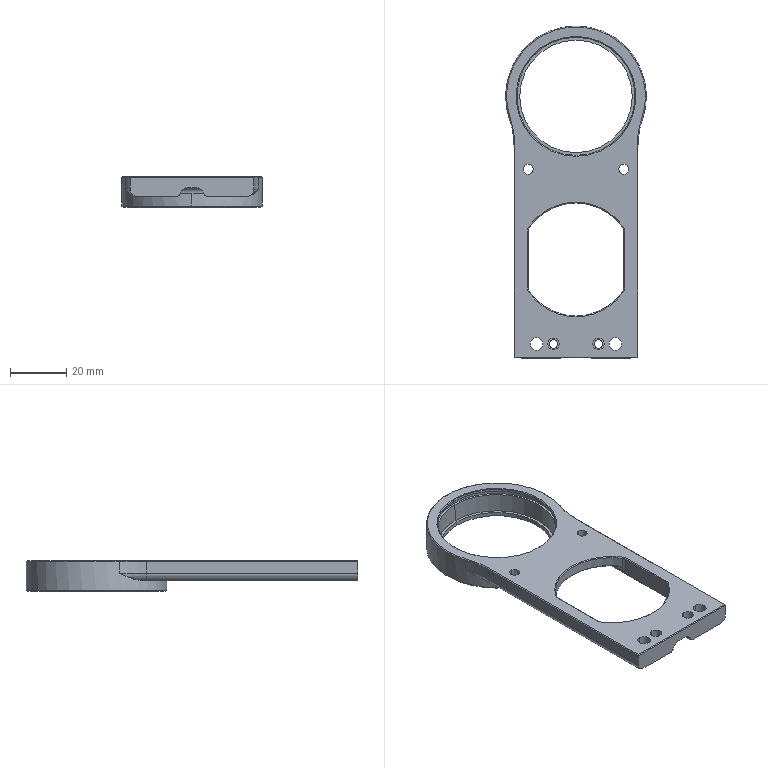NC program | NX | posted with a generic post | part box 50 x 118 x 11 mm
Lines 1103 to 2100 of 9841:
(ZLEVEL_PROFILE_1_COPY , TOOL : D3R0.5)
N2168 T18 M6
N2170 G54
N2172 G17 G0 G90 X65.824 Y-6.743 S9500 M3
N2174 G43 Z30. H18
N2176 Z-1.012
N2178 G94 G1 Z-4.012 F1000.
N2180 X65.888 Y-6.726
N2182 G3 X66.956 Y-4.893 R1.5
N2184 G2 X66.711 Y-3.914 R38.728 F2500.
N2186 G1 X66.672 Y-3.67
N2188 X66.526 Y-2.446
N2190 X66.5 Y-2.202
N2192 X66.495 Y-2.079
N2194 X66.436 Y-0.489
N2196 X66.429 Y-0.245
N2198 X66.5 Y2.202
N2200 X66.526 Y2.446
N2202 X66.663 Y3.595
N2204 G2 X66.812 Y4.34 R4.831
N2206 G3 X67.039 Y5.31 R10.605
N2208 G1 X67.047 Y5.352 Z-4.025
N2210 G2 X66.812 Y4.342 R11.706
N2212 G3 X66.662 Y3.59 R4.971
N2214 G1 X66.526 Y2.446
N2216 X66.5 Y2.202
N2218 X66.429 Y-0.245
N2220 X66.436 Y-0.489
N2222 X66.495 Y-2.079
N2224 X66.5 Y-2.202
N2226 X66.526 Y-2.446
N2228 X66.672 Y-3.67
N2230 X66.711 Y-3.914
N2232 G3 X66.956 Y-4.893 R23.385
N2234 G1 X66.971 Y-4.975 Z-4.03
N2236 X66.987 Y-5.056 Z-4.034
N2238 X67.003 Y-5.138 Z-4.039
N2240 G3 X66.837 Y-4.45 R8.75
N2242 G2 X66.658 Y-3.557 R5.791
N2244 G1 X66.526 Y-2.446
N2246 X66.5 Y-2.202
N2248 X66.495 Y-2.079
N2250 X66.436 Y-0.489
N2252 X66.429 Y-0.245
N2254 X66.5 Y2.202
N2256 X66.526 Y2.446
N2258 X66.672 Y3.67
N2260 X66.711 Y3.914
N2262 G2 X66.953 Y4.893 R19.424
N2264 G1 X67.056 Y5.396
N2266 X67.069 Y5.454 Z-4.057
N2268 G2 X66.829 Y4.433 R13.052
N2270 G3 X66.663 Y3.593 R5.641
N2272 G1 X66.526 Y2.446
N2274 X66.5 Y2.202
N2276 X66.429 Y-0.245
N2278 X66.436 Y-0.489
N2280 X66.495 Y-2.079
N2282 X66.5 Y-2.202
N2284 X66.526 Y-2.446
N2286 X66.664 Y-3.605
N2288 G3 X66.82 Y-4.399 R5.379
N2290 G2 X67.003 Y-5.138 R13.895
N2292 G1 Z-4.08
N2294 G2 X66.711 Y-3.914 R40.513
N2296 G1 X66.672 Y-3.67
N2298 X66.526 Y-2.446
N2300 X66.5 Y-2.202
N2302 X66.495 Y-2.079
N2304 X66.436 Y-0.489
N2306 X66.429 Y-0.245
N2308 X66.5 Y2.202
N2310 X66.526 Y2.446
N2312 X66.672 Y3.67
N2314 X66.711 Y3.914
N2316 X66.895 Y4.704
N2318 X66.946 Y4.893
N2320 X67.084 Y5.528
N2322 X67.104 Y5.618 Z-4.108
N2324 X67.002 Y5.138
N2326 G3 X66.711 Y3.914 R30.653
N2328 G1 X66.672 Y3.67
N2330 X66.526 Y2.446
N2332 X66.5 Y2.202
N2334 X66.429 Y-0.245
N2336 X66.436 Y-0.489
N2338 X66.495 Y-2.079
N2340 X66.5 Y-2.202
N2342 X66.526 Y-2.446
N2344 X66.665 Y-3.614
N2346 G3 X66.788 Y-4.271 R5.109
N2348 G2 X67.052 Y-5.382 R35.004
N2350 G1 Z-4.141
N2352 G2 X66.711 Y-3.914 R82.106
N2354 G1 X66.672 Y-3.67
N2356 X66.526 Y-2.446
N2358 X66.5 Y-2.202
N2360 X66.495 Y-2.079
N2362 X66.436 Y-0.489
N2364 X66.429 Y-0.245
N2366 X66.5 Y2.202
N2368 X66.526 Y2.446
N2370 X66.672 Y3.67
N2372 X66.711 Y3.914
N2374 G2 X67.027 Y5.26 R42.81
N2376 G1 X67.127 Y5.726
N2378 X67.14 Y5.79 Z-4.161
N2380 X67.156 Y5.854 Z-4.182
N2382 G3 X66.711 Y3.914 R511.613
N2384 G1 X66.672 Y3.67
N2386 X66.526 Y2.446
N2388 X66.5 Y2.202
N2390 X66.429 Y-0.245
N2392 X66.436 Y-0.489
N2394 X66.495 Y-2.079
N2396 X66.5 Y-2.202
N2398 X66.526 Y-2.446
N2400 X66.672 Y-3.67
N2402 X66.711 Y-3.914
N2404 X67.104 Y-5.627
N2406 Z-4.228
N2408 X67.046 Y-5.382
N2410 X66.711 Y-3.914
N2412 X66.672 Y-3.67
N2414 X66.525 Y-2.446
N2416 X66.5 Y-2.202
N2418 X66.495 Y-2.079
N2420 X66.436 Y-0.489
N2422 X66.429 Y-0.245
N2424 X66.5 Y2.202
N2426 X66.525 Y2.446
N2428 X66.672 Y3.67
N2430 X66.711 Y3.914
N2432 X67.19 Y6.003
N2434 X67.216 Y6.119 Z-4.232
N2436 X67.244 Y6.235 Z-4.236
N2438 X67.272 Y6.35 Z-4.24
N2440 X67.301 Y6.465 Z-4.244
N2442 X67.33 Y6.581 Z-4.248
N2444 X67.36 Y6.696 Z-4.252
N2446 X67.39 Y6.811 Z-4.256
N2448 X67.421 Y6.926 Z-4.26
N2450 X67.452 Y7.04 Z-4.264
N2452 X67.484 Y7.155 Z-4.268
N2454 X67.516 Y7.269 Z-4.272
N2456 X67.549 Y7.383 Z-4.276
N2458 X67.584 Y7.497 Z-4.28
N2460 X67.562 Y7.429
N2462 G3 X67.275 Y6.361 R26.5
N2464 G1 X67.229 Y6.17
N2466 X66.711 Y3.914
N2468 X66.672 Y3.67
N2470 X66.525 Y2.446
N2472 X66.5 Y2.202
N2474 X66.429 Y-0.245
N2476 X66.436 Y-0.489
N2478 X66.495 Y-2.079
N2480 X66.5 Y-2.202
N2482 X66.525 Y-2.446
N2484 X66.672 Y-3.67
N2486 X66.711 Y-3.914
N2488 X67.1 Y-5.627
N2490 X67.139 Y-5.786
N2492 X67.164 Y-5.896 Z-4.3
N2494 X67.19 Y-6.006 Z-4.319
N2496 X67.215 Y-6.116 Z-4.338
N2498 X67.139 Y-5.806
N2500 X66.711 Y-3.914
N2502 X66.672 Y-3.67
N2504 X66.525 Y-2.446
N2506 X66.5 Y-2.202
N2508 X66.494 Y-2.079
N2510 X66.436 Y-0.489
N2512 X66.429 Y-0.245
N2514 X66.5 Y2.202
N2516 X66.525 Y2.446
N2518 X66.672 Y3.67
N2520 X66.711 Y3.914
N2522 X67.156 Y5.872
N2524 X67.273 Y6.356
N2526 G2 X67.562 Y7.429 R26.5
N2528 G1 X67.689 Y7.843
N2530 X67.724 Y7.958 Z-4.357
N2532 X67.759 Y8.072 Z-4.376
N2534 X67.798 Y8.186 Z-4.396
N2536 X67.761 Y8.073
N2538 X67.562 Y7.429
N2540 G3 X67.401 Y6.85 R26.5
N2542 G1 X67.211 Y6.116
N2544 X66.711 Y3.914
N2546 X66.672 Y3.67
N2548 X66.525 Y2.446
N2550 X66.5 Y2.202
N2552 X66.429 Y-0.245
N2554 X66.436 Y-0.489
N2556 X66.494 Y-2.079
N2558 X66.5 Y-2.202
N2560 X66.525 Y-2.446
N2562 X66.679 Y-3.728
N2564 X66.711 Y-3.914
N2566 X66.821 Y-4.404
N2568 G3 X67.401 Y-6.85 R55.508
N2570 G2 X66.375 Y-8.667 R1.5
N2572 G1 Z-1.396
N2574 G0 Z30.
N2576 X66.98 Y10.342
N2578 Z-1.012
N2580 G1 Z-4.012 F1000.
N2582 X67.069 Y10.67
N2584 G3 X69.068 Y11.38 R1.5
N2586 X68.117 Y11.815 R1.175 F2500.
N2588 G2 X66.766 Y11.857 R19.276
N2590 X62.407 Y14.841 R5.188
N2592 G1 X62.15 Y15.393
N2594 G3 X61.116 Y16.058 R1.153
N2596 X55.407 Y16.081 R499.96
N2598 G1 X19.231
N2600 G3 X16.054 Y16.067 R245.525
N2602 X13.825 Y15.413 R4.23
N2604 X11.961 Y12.304 R4.024
N2606 G1 X11.948 Y12.12
N2608 X11.941 Y11.98
N2610 G3 X11.912 Y8.807 R243.377
N2612 G2 X11.873 Y5.627 R132.454
N2614 X11.41 Y4.456 R1.784
N2616 G1 X11.349 Y4.404
N2618 X10.823 Y4.199
N2620 X10.7 Y4.183
N2622 X0.
N2624 X-0.567 Y4.264
N2626 X-1.301 Y4.266
N2628 X-5.507 Y4.267
N2630 X-5.505 Y4.206 Z-4.025
N2632 X-1.114 Y4.216
N2634 G2 X0. Y4.1 R5.322
N2636 G1 X10.702
N2638 G3 X11.711 Y4.765 R1.098
N2640 X11.899 Y5.623 R2.317
N2642 X11.947 Y11.908 R1667.102
N2644 G2 X11.985 Y12.477 R4.694
N2646 X13.365 Y15.06 R4.118
N2648 X16.054 Y16.055 R4.192
N2650 G1 X19.231 Y16.068
N2652 X55.407
N2654 G2 X61.114 Y16.047 R541.797
N2656 X62.141 Y15.383 R1.142
N2658 G1 X62.384 Y14.856
N2660 G3 X66.773 Y11.842 R5.199
N2662 X68.117 Y11.803 R19.126
N2664 G2 X69.05 Y11.387 R1.177
N2666 G1 X69.069 Y11.377
N2668 Y11.357
N2670 X69.052 Y11.346
N2672 Z-4.039
N2674 X69.051 Y11.366
N2676 X68.947 Y11.482
N2678 G3 X68.117 Y11.791 R1.169
N2680 G2 X66.764 Y11.827 R17.391
N2682 X62.237 Y15.16 R5.219
N2684 G3 X61.835 Y15.775 R1.746
N2686 X61.102 Y16.036 R1.185
N2688 G1 X59.073 Y16.05
N2690 X58.584 Y16.051
N2692 X57.118 Y16.053
N2694 X17.52
N2696 X16.054 Y16.043
N2698 G3 X12.994 Y14.679 R4.149
N2700 X11.961 Y11.988 R4.139
N2702 X11.922 Y5.692 R2205.64
N2704 G2 X11.825 Y4.95 R2.986
N2706 X10.7 Y4.034 R1.228
N2708 G1 X0.
N2710 G3 X-0.832 Y4.153 R3.146
N2712 G1 X-2.034 Y4.163
N2714 X-5.502 Y4.146
N2716 Y4.105 Z-4.048
N2718 Y4.09 Z-4.057
N2720 X-1.08 Y4.106
N2722 G2 X0. Y3.964 R4.091
N2724 G1 X10.7
N2726 G3 X11.935 Y5.292 R1.341
N2728 G1 X11.977 Y11.988
N2730 G2 X16.054 Y16.027 R4.073
N2732 G1 X17.52 Y16.035
N2734 X59.073 Y16.033
N2736 X61.126 Y16.02
N2738 G2 X61.962 Y15.611 R1.072
N2740 X62.208 Y15.168 R1.589
N2742 G3 X66.895 Y11.798 R5.257
N2744 X68.117 Y11.774 R18.624
N2746 G2 X69.039 Y11.36 R1.133
N2748 G1 X69.056 Y11.344
N2750 X69.042 Y11.325
N2752 X69.031 Y11.303 Z-4.08
N2754 X69.039 Y11.323
N2756 X69.016 Y11.359
N2758 G3 X68.117 Y11.753 R1.154
N2760 G2 X66.79 Y11.78 R16.906
N2762 X62.182 Y15.168 R5.259
N2764 G3 X61.835 Y15.721 R1.362
N2766 X61.147 Y16.001 R0.997
N2768 G1 X59.073 Y16.011
N2770 X17.52 Y16.012
N2772 X16.054 Y16.006
N2774 G3 X11.998 Y11.988 R4.04
N2776 G1 X11.995 Y11.743
N2778 X11.971 Y5.378
N2780 G2 X11.425 Y4.149 R1.559
N2782 X10.725 Y3.891 R1.078
N2784 G1 X0.
N2786 G3 X-1.199 Y4.031 R5.058
N2788 G1 X-5.501 Y4.017
N2790 Y3.964 Z-4.094
N2792 Y3.928 Z-4.108
N2794 X-1.079 Y3.945
N2796 G2 X0. Y3.815 R4.388
N2798 G1 X10.718
N2800 G3 X11.597 Y4.222 R1.154
N2802 X12.009 Y5.375 R1.732
N2804 G1 X12.023 Y11.988
N2806 G2 X16.054 Y15.981 R4.009
N2808 G1 X61.121 Y15.977
N2810 G2 X62.068 Y15.357 R1.033
N2812 G1 X62.15 Y15.168
N2814 G3 X66.802 Y11.748 R5.275
N2816 G1 X66.899 Y11.743
N2818 X68.204 Y11.727
N2820 G2 X69.013 Y11.326 R1.041
N2822 G1 X69.033 Y11.303
N2824 X69.018 Y11.275
N2826 X69.016 Y11.269 Z-4.141
N2828 G3 X68.211 Y11.695 R1.011
N2830 X67.141 Y11.7 R36.581
N2832 G2 X62.112 Y15.168 R5.307
N2834 G1 X62.037 Y15.348
N2836 G3 X61.135 Y15.949 R0.978
N2838 G1 X16.054 Y15.951
N2840 G3 X12.053 Y11.988 R3.972
N2842 G1 X12.05 Y11.743
N2844 X12.048 Y5.382
N2846 G2 X11.695 Y4.248 R1.843
N2848 X10.7 Y3.737 R1.243
N2850 G1 X0.
N2852 X-0.567 Y3.849
N2854 X-1.545 Y3.86
N2856 X-5.501 Y3.85
N2858 Y3.804 Z-4.161
N2860 Y3.762 Z-4.182
N2862 X-1.301 Y3.764
N2864 X-0.567 Y3.759
N2866 X-0.078 Y3.661
N2868 X0. Y3.658
N2870 X10.703
N2872 G3 X11.725 Y4.187 R1.251
N2874 X12.089 Y5.373 R1.988
N2876 G1 Y12.
N2878 G2 X16. Y15.911 R3.911
N2880 G1 X61.162
N2882 G2 X62.026 Y15.292 R0.911
N2884 G3 X67.084 Y11.661 R5.339
N2886 G1 X68.232
N2888 G2 X68.978 Y11.274 R0.911
N2890 G1 X68.998 Y11.233
N2892 X68.978 Y11.189 Z-4.228
N2894 G3 X68.232 Y11.615 R0.865
N2896 G1 X67.084
N2898 G2 X61.982 Y15.277 R5.385
N2900 G3 X61.162 Y15.865 R0.865
N2902 G1 X16.
N2904 G3 X12.135 Y12. R3.865
N2906 G1 Y5.373
N2908 G2 X11.899 Y4.356 R2.322
N2910 X10.7 Y3.578 R1.375
N2912 G1 X0.
N2914 X-0.078 Y3.583
N2916 X-0.567 Y3.661
N2918 X-5.501 Y3.663
N2920 Y3.619 Z-4.254
N2922 Y3.591 Z-4.28
N2924 X-5.456 Y3.588
N2926 X-0.567
N2928 X-0.078 Y3.505
N2930 X0. Y3.5
N2932 X10.7
N2934 G3 X11.844 Y4.159 R1.37
N2936 X12.187 Y5.373 R2.425
N2938 G1 Y12.
N2940 G2 X16. Y15.813 R3.813
N2942 G1 X61.162
N2944 G2 X61.932 Y15.26 R0.813
N2946 G3 X67.084 Y11.563 R5.437
N2948 G1 X68.232
N2950 G2 X68.951 Y11.13 R0.813
N2952 G1 X68.919 Y11.062 Z-4.338
N2954 G3 X68.232 Y11.505 R0.755
N2956 G1 X67.084
N2958 G2 X61.877 Y15.242 R5.495
N2960 G3 X61.162 Y15.755 R0.755
N2962 G1 X16.
N2964 G3 X12.245 Y12. R3.755
N2966 G1 Y5.373
N2968 G2 X11.908 Y4.159 R2.655
N2970 X10.7 Y3.424 R1.41
N2972 G1 X0.
N2974 X-0.078 Y3.427
N2976 X-0.567 Y3.508
N2978 X-5.456
N2980 X-5.501 Y3.511
N2982 X-5.5 Y3.465 Z-4.367
N2984 Y3.431 Z-4.396
N2986 X-5.456 Y3.428
N2988 X-0.567
N2990 X-0.078 Y3.364
N2992 X0. Y3.358
N2994 X10.7
N2996 G3 X11.899 Y4.056 R1.424
N2998 G1 X11.954 Y4.159
N3000 G3 X12.303 Y5.373 R2.541
N3002 G1 Y12.
N3004 G2 X16. Y15.697 R3.697
N3006 G1 X61.162
N3008 G2 X61.823 Y15.223 R0.697
N3010 G3 X67.084 Y11.447 R5.553
N3012 G1 X68.232
N3014 G2 X68.887 Y10.991 R0.697
N3016 G1 Z-1.396
N3018 G0 Z30.
N3020 X66.657 Y-9.491
N3022 Z-1.463
N3024 G1 Z-4.463 F1000.
N3026 X66.67 Y-9.486
N3028 G3 X67.608 Y-7.584 R1.5
N3030 G2 X67.267 Y-6.361 R11.656 F2500.
N3032 G1 X66.711 Y-3.914
N3034 X66.672 Y-3.67
N3036 X66.525 Y-2.446
N3038 X66.499 Y-2.202
N3040 X66.494 Y-2.079
N3042 X66.436 Y-0.489
N3044 X66.429 Y-0.245
N3046 X66.499 Y2.202
N3048 X66.525 Y2.446
N3050 X66.672 Y3.67
N3052 X66.711 Y3.914
N3054 X67.267 Y6.361
N3056 X67.324 Y6.605
N3058 G2 X67.563 Y7.439 R7.345
N3060 G1 X67.608 Y7.584
N3062 X67.628 Y7.65
N3064 X67.873 Y8.417
N3066 X67.932 Y8.587
N3068 G2 X68.63 Y10.409 R25.949
N3070 X68.845 Y10.898 R26.5
N3072 G3 X68.243 Y11.38 R0.63
N3074 G1 X67.074
N3076 G2 X61.759 Y15.202 R5.62
N3078 G3 X61.162 Y15.63 R0.63
N3080 G1 X16.
N3082 G3 X12.37 Y12. R3.63
N3084 G1 Y5.382
N3086 G2 X11.712 Y3.736 R2.641
N3088 X10.722 Y3.289 R1.32
N3090 G1 X0.
N3092 X-0.078 Y3.292
N3094 X-0.567 Y3.353
N3096 X-5.456
N3098 X-5.501 Y3.356
N3100 Y3.318 Z-4.499
N3102 Y3.286 Z-4.534
N3104 X-5.456 Y3.284
N3106 X-0.567
N3108 X0. Y3.225
N3110 X10.701
N3112 G3 X11.707 Y3.659 R1.383
N3114 X12.065 Y4.159 R2.282
N3116 X12.423 Y5.382 R2.238
N3118 G1 Y12.
N3120 G2 X16. Y15.577 R3.577
N3122 G1 X61.162
N3124 G2 X61.708 Y15.184 R0.577
N3126 G3 X67.077 Y11.327 R5.673
N3128 G1 X67.091 Y11.33
N3130 X68.239 Y11.326
N3132 G2 X68.806 Y10.811 R0.577
N3134 G3 X68.702 Y10.576 R26.5
N3136 X68.015 Y8.828 R24.512
N3138 X67.602 Y7.584 R49.71
N3140 G1 X67.547 Y7.434
N3142 X67.518 Y7.398
N3144 X67.514 Y7.351
N3146 X67.505 Y7.339
N3148 X67.44 Y7.095
N3150 X67.384 Y6.877
N3152 X66.711 Y3.914
N3154 X66.672 Y3.67
N3156 X66.525 Y2.446
N3158 X66.499 Y2.202
N3160 X66.429 Y-0.245
N3162 X66.436 Y-0.489
N3164 X66.494 Y-2.079
N3166 X66.499 Y-2.202
N3168 X66.525 Y-2.446
N3170 X66.672 Y-3.67
N3172 X66.711 Y-3.914
N3174 X67.366 Y-6.798
N3176 G3 X67.51 Y-7.339 R7.568
N3178 G1 X67.683 Y-7.829
N3180 X67.705 Y-7.901 Z-4.605
N3182 X67.681 Y-7.829
N3184 X67.498 Y-7.339
N3186 G2 X67.385 Y-6.886 R11.568
N3188 G1 X66.711 Y-3.914
N3190 X66.672 Y-3.67
N3192 X66.525 Y-2.446
N3194 X66.499 Y-2.202
N3196 X66.494 Y-2.079
N3198 X66.436 Y-0.489
N3200 X66.429 Y-0.245
N3202 X66.499 Y2.202
N3204 X66.525 Y2.446
N3206 X66.672 Y3.67
N3208 X66.711 Y3.914
N3210 X67.454 Y7.186
N3212 G2 X67.517 Y7.392 R1.483
N3214 G1 X67.591 Y7.584
N3216 X68.03 Y8.871
N3218 G2 X68.702 Y10.576 R25.923
N3220 G1 X68.772 Y10.735
N3222 G3 X68.24 Y11.29 R0.54
N3224 G1 X67.075
N3226 G2 X61.673 Y15.173 R5.71
N3228 G3 X61.162 Y15.54 R0.54
N3230 G1 X16.
N3232 G3 X12.46 Y12. R3.54
N3234 G1 Y5.325
N3236 G2 X12.148 Y4.199 R2.186
N3238 X11.817 Y3.716 R4.915
N3240 X10.701 Y3.169 R1.413
N3242 G1 X0.
N3244 X-0.078 Y3.173
N3246 X-0.567 Y3.23
N3248 X-5.456
N3250 X-5.501 Y3.233
N3252 G3 X-7.024 Y2.167 R1.5
N3254 G1 Z-1.605
N3256 G0 Z30.
N3258 X-6.945 Y-3.221
N3260 Z-1.012
N3262 G1 Z-4.012 F1000.
N3264 G3 X-5.51 Y-4.274 R1.5
N3266 G1 X-0.567 Y-4.265 F2500.
N3268 X0. Y-4.183
N3270 X10.7
N3272 G2 X11.809 Y-5.277 R1.245
N3274 G1 Y-6.018
N3276 Y-6.308
N3278 G3 X11.88 Y-6.85 R2.064
N3280 G1 X11.892 Y-7.095
N3282 Y-8.318
N3284 G3 X11.929 Y-11.988 R205.161
N3286 X12.632 Y-14.245 R4.237
N3288 X15.809 Y-16.047 R4.056
N3290 G1 X16.054 Y-16.063
N3292 X17.52 Y-16.072
N3294 X18.009 Y-16.077
N3296 X59.806
N3298 X61.029 Y-16.065
N3300 G3 X61.762 Y-15.854 R1.26
N3302 G1 X61.924 Y-15.705
N3304 G3 X62.129 Y-15.425 R0.907
N3306 G1 X62.406 Y-14.837
N3308 G2 X62.784 Y-14.168 R5.244
N3310 X66.997 Y-11.848 R5.205
N3312 G1 X68.117 Y-11.822
N3314 G3 X69.06 Y-11.391 R1.208
N3316 G1 X69.062 Y-11.367
N3318 Z-4.025
N3320 G2 X68.117 Y-11.81 R1.174
N3322 G1 X67.139 Y-11.828
N3324 G3 X65.685 Y-12.032 R5.572
N3326 X62.403 Y-14.811 R5.149
N3328 G1 X62.122 Y-15.413
N3330 G2 X61.762 Y-15.841 R1.326
N3332 X61.029 Y-16.053 R1.247
N3334 G1 X57.851 Y-16.068
N3336 X17.765 Y-16.062
N3338 X17.032 Y-16.056
N3340 X16.016 Y-16.05
N3342 G2 X15.809 Y-16.035 R1.661
N3344 X12.337 Y-13.7 R4.048
N3346 X11.941 Y-11.988 R4.292
N3348 X11.908 Y-7.095 R218.224
N3350 G3 X11.856 Y-6.605 R2.042
N3352 G1 Y-6.147
N3354 Y-5.334
N3356 G3 X10.7 Y-4.1 R1.228
N3358 G1 X0.
N3360 X-0.567 Y-4.207
N3362 X-5.503 Y-4.2
N3364 X-5.502 Y-4.156 Z-4.032
N3366 Y-4.137 Z-4.039
N3368 X-5.211 Y-4.15
N3370 X-1.056 Y-4.16
N3372 X-0.567 Y-4.149
N3374 X0. Y-4.034
N3376 X10.7
N3378 G2 X11.893 Y-5.31 R1.29
N3380 G1 Y-6.605
N3382 X11.924 Y-7.095
N3384 G3 X11.954 Y-11.988 R240.726
N3386 X12.994 Y-14.679 R4.199
N3388 X15.809 Y-16.024 R4.04
N3390 G1 X15.907 Y-16.044
N3392 X16.007 Y-16.038
N3394 X18.009 Y-16.051
N3396 X59.806
N3398 X61.102 Y-16.041
N3400 G3 X62.122 Y-15.383 R1.134
N3402 G1 X62.448 Y-14.679
N3404 X62.493 Y-14.594
N3406 G2 X67.009 Y-11.818 R5.221
N3408 G1 X68.117 Y-11.798
N3410 G3 X68.947 Y-11.481 R1.203
N3412 G1 X69.054 Y-11.361
N3414 X69.052 Y-11.346
N3416 X69.042 Y-11.325 Z-4.057
N3418 X69.056 Y-11.343
N3420 X69.039 Y-11.359
N3422 G2 X68.117 Y-11.781 R1.154
N3424 G1 X67.01 Y-11.799
N3426 G3 X62.561 Y-14.439 R5.208
N3428 X62.118 Y-15.346 R8.257
N3430 G2 X61.109 Y-16.025 R1.1
N3432 G1 X59.806 Y-16.033
N3434 X17.765 Y-16.031
N3436 X16.298 Y-16.024
N3438 G2 X15.728 Y-16.005 R7.392
N3440 X11.989 Y-12.259 R4.035
N3442 G1 X11.971 Y-11.988
N3444 X11.957 Y-10.275
N3446 X11.949 Y-9.786
N3448 X11.946 Y-7.095
N3450 X11.931 Y-6.727
N3452 Y-5.299
N3454 G3 X10.7 Y-3.964 R1.339
N3456 G1 X0.
N3458 X-0.567 Y-4.091
N3460 X-1.056 Y-4.102
N3462 X-5.211 Y-4.094
N3464 X-5.502 Y-4.079
N3466 Y-4.024 Z-4.068
N3468 X-5.501 Y-4.005 Z-4.08
N3470 X-5.211 Y-4.023
N3472 X-1.301 Y-4.033
N3474 X-0.567 Y-4.016
N3476 X0. Y-3.891
N3478 X10.7
N3480 G2 X11.813 Y-4.648 R1.255
N3482 X11.971 Y-5.382 R1.87
N3484 G1 Y-6.728
N3486 X11.992 Y-11.988
N3488 G3 X16.054 Y-16.004 R4.049
N3490 G1 X18.009 Y-16.011
N3492 X59.562 Y-16.012
N3494 X61.116 Y-16.005
N3496 G3 X62.097 Y-15.34 R1.063
N3498 G2 X62.547 Y-14.412 R7.701
N3500 X67.053 Y-11.769 R5.238
N3502 G1 X68.166 Y-11.76
N3504 G3 X69.028 Y-11.343 R1.119
N3506 G1 X69.046 Y-11.324
N3508 X69.031 Y-11.303
N3510 X69.018 Y-11.275 Z-4.108
N3512 X69.027 Y-11.299
N3514 X68.999 Y-11.342
N3516 G2 X68.117 Y-11.734 R1.118
N3518 G1 X67.066 Y-11.738
N3520 G3 X62.276 Y-14.876 R5.257
N3522 G1 X62.061 Y-15.364
N3524 G2 X61.116 Y-15.981 R1.032
N3526 G1 X16.054 Y-15.979
N3528 G2 X12.019 Y-11.988 R4.015
N3530 G1 X12.006 Y-6.743
N3532 X12.01 Y-6.728
N3534 Y-5.374
N3536 G3 X11.868 Y-4.648 R2.215
N3538 X10.7 Y-3.815 R1.303
N3540 G1 X0.
N3542 X-0.567 Y-3.925
N3544 X-1.301 Y-3.944
N3546 X-5.211 Y-3.935
N3548 X-5.501 Y-3.913
N3550 Y-3.876 Z-4.125
N3552 Y-3.843 Z-4.141
N3554 X-5.211 Y-3.853
N3556 X-1.301 Y-3.857
N3558 X-0.567 Y-3.847
N3560 X0. Y-3.737
N3562 X10.7
N3564 G2 X11.899 Y-4.595 R1.349
N3566 X12.048 Y-5.381 R2.172
N3568 G1 Y-6.729
N3570 X12.047 Y-6.744
N3572 X12.049 Y-11.743
N3574 X12.051 Y-11.988
N3576 G3 X16.054 Y-15.949 R3.975
N3578 G1 X61.131 Y-15.951
N3580 G3 X62.039 Y-15.325 R0.972
N3582 G2 X62.529 Y-14.303 R6.754
N3584 X67.205 Y-11.704 R5.271
N3586 G3 X68.361 Y-11.683 R13.604
N3588 X69.016 Y-11.269 R1.047
N3590 G1 X68.998 Y-11.233 Z-4.182
N3592 X68.968 Y-11.279
N3594 X68.966 Y-11.29
N3596 G2 X68.826 Y-11.441 R0.911
N3598 X68.232 Y-11.661 R0.911
N3600 G1 X67.084
N3602 G3 X62.026 Y-15.292 R5.339
N3604 G2 X61.162 Y-15.911 R0.911
N3606 G1 X16.
N3608 G2 X12.089 Y-12. R3.911
N3610 G1 Y-5.373
N3612 G3 X11.864 Y-4.404 R2.172
N3614 X10.7 Y-3.658 R1.352
N3616 G1 X0.
N3618 X-0.078 Y-3.661
N3620 X-0.567 Y-3.758
N3622 X-5.211 Y-3.761
N3624 X-5.501 Y-3.758
N3626 Y-3.706 Z-4.205
N3628 Y-3.663 Z-4.228
N3630 X-0.567 Y-3.661
N3632 X0. Y-3.578
N3634 X10.7
N3636 G2 X11.899 Y-4.356 R1.375
N3638 X12.135 Y-5.373 R2.322
N3640 G1 Y-12.
N3642 G3 X16.005 Y-15.865 R3.865
N3644 G1 X61.162
N3646 G3 X61.982 Y-15.277 R0.865
N3648 G2 X67.084 Y-11.615 R5.385
N3650 G1 X68.232
N3652 G3 X68.978 Y-11.189 R0.865
N3654 G1 X68.951 Y-11.13 Z-4.28
N3656 G2 X68.232 Y-11.563 R0.813
N3658 G1 X67.084
N3660 G3 X61.932 Y-15.26 R5.437
N3662 G2 X61.162 Y-15.813 R0.813
N3664 G1 X16.
N3666 G2 X12.187 Y-12. R3.813
N3668 G1 Y-5.373
N3670 G3 X11.844 Y-4.159 R2.429
N3672 X10.7 Y-3.5 R1.37
N3674 G1 X0.
N3676 X-0.078 Y-3.505
N3678 X-0.567 Y-3.588
N3680 X-5.456
N3682 X-5.501 Y-3.591
N3684 Y-3.54 Z-4.309
N3686 Y-3.511 Z-4.338
N3688 X-5.456 Y-3.508
N3690 X-0.567
N3692 X-0.025 Y-3.425
N3694 X10.7 Y-3.424
N3696 G2 X11.908 Y-4.159 R1.41
N3698 X12.245 Y-5.373 R2.69
N3700 G1 Y-12.
N3702 G3 X16.003 Y-15.755 R3.755
N3704 G1 X61.162
N3706 G3 X61.877 Y-15.242 R0.755
N3708 G2 X67.084 Y-11.505 R5.495
N3710 G1 X68.232
N3712 G3 X68.919 Y-11.062 R0.755
N3714 G1 X68.887 Y-10.991 Z-4.396
N3716 G2 X68.232 Y-11.447 R0.697
N3718 G1 X67.084
N3720 G3 X61.823 Y-15.223 R5.553
N3722 G2 X61.162 Y-15.697 R0.697
N3724 G1 X16.
N3726 G2 X12.303 Y-12. R3.697
N3728 G1 Y-5.373
N3730 G3 X11.798 Y-3.914 R2.655
N3732 X10.7 Y-3.358 R1.397
N3734 G1 X0.
N3736 X-0.567 Y-3.428
N3738 X-5.456
N3740 X-5.5 Y-3.431
N3742 X-5.501 Y-3.385 Z-4.43
N3744 Y-3.356 Z-4.463
N3746 X-5.456 Y-3.353
N3748 X-0.567
N3750 X0. Y-3.289
N3752 X10.723
N3754 G2 X11.716 Y-3.741 R1.317
N3756 X12.37 Y-5.382 R2.668
N3758 G1 Y-12.
N3760 G3 X16. Y-15.63 R3.63
N3762 G1 X61.162
N3764 G3 X61.759 Y-15.202 R0.63
N3766 G2 X67.084 Y-11.38 R5.62
N3768 G1 X68.232
N3770 G3 X68.845 Y-10.898 R0.63
N3772 G1 X68.806 Y-10.811 Z-4.534
N3774 G2 X68.232 Y-11.327 R0.577
N3776 G1 X67.084
N3778 G3 X61.708 Y-15.184 R5.673
N3780 G2 X61.162 Y-15.577 R0.577
N3782 G1 X16.
N3784 G2 X12.423 Y-12. R3.577
N3786 G1 Y-5.382
N3788 X12.387 Y-4.959
N3790 G3 X11.718 Y-3.67 R2.943
N3792 X10.7 Y-3.225 R1.403
N3794 G1 X0.
N3796 X-0.567 Y-3.284
N3798 X-5.456
N3800 X-5.501 Y-3.286
N3802 Y-3.257 Z-4.57
N3804 Y-3.233 Z-4.605
N3806 X-5.456 Y-3.23
N3808 X-0.567
N3810 G2 X0. Y-3.169 R59.732
N3812 G1 X10.701
N3814 G2 X11.817 Y-3.716 R1.413
N3816 X12.143 Y-4.19 R4.911
N3818 X12.46 Y-5.331 R2.208
N3820 G1 Y-12.
N3822 G3 X16. Y-15.54 R3.54
N3824 G1 X61.162
N3826 G3 X61.673 Y-15.173 R0.54
N3828 G2 X67.084 Y-11.29 R5.71
N3830 G1 X68.232
N3832 G3 X68.772 Y-10.735 R0.54
N3834 X66.793 Y-9.971 R1.5
N3836 G1 X66.77 Y-9.796
N3838 Z-1.605
N3840 G0 Z30.
N3842 X-7.018 Y2.1
N3844 Z-1.683
N3846 G1 Z-4.683 F1000.
N3848 G2 X-5.5 Y3.173 R1.5
N3850 G1 X-5.456 Y3.171 F2500.
N3852 X-0.567
N3854 X0. Y3.115
N3856 X10.7
N3858 G3 X11.899 Y3.76 R1.469
N3860 X12.387 Y4.591 R2.668
N3862 X12.486 Y5.382 R3.074
N3864 G1 Y12.
N3866 G2 X16. Y15.514 R3.514
N3868 G1 X61.162
N3870 G2 X61.649 Y15.164 R0.514
N3872 G3 X67.084 Y11.264 R5.736
N3874 G1 X68.232
N3876 G2 X68.738 Y10.659 R0.514
N3878 G1 X68.702 Y10.576
N3880 X68.41 Y9.873
N3882 X68.358 Y9.745
N3884 X68.047 Y8.918
N3886 X67.677 Y7.829
N3888 X67.566 Y7.536
N3890 G3 X67.434 Y7.098 R3.306
N3892 G1 X66.711 Y3.914
N3894 X66.672 Y3.67
N3896 X66.525 Y2.446
N3898 X66.499 Y2.202
N3900 X66.429 Y-0.245
N3902 X66.436 Y-0.489
N3904 X66.494 Y-2.079
N3906 X66.499 Y-2.202
N3908 X66.525 Y-2.446
N3910 X66.672 Y-3.67
N3912 X66.711 Y-3.914
N3914 X67.385 Y-6.886
N3916 G3 X67.498 Y-7.339 R11.617
N3918 G2 X67.868 Y-8.401 R23.776
N3920 G3 X68.688 Y-10.545 R26.356
N3922 G1 X68.738 Y-10.659
N3924 G2 X68.232 Y-11.264 R0.514
N3926 G1 X67.084
N3928 G3 X61.649 Y-15.164 R5.736
N3930 G2 X61.162 Y-15.514 R0.514
N3932 G1 X16.
N3934 G2 X12.486 Y-12. R3.514
N3936 G1 Y-5.382
N3938 G3 X12.387 Y-4.591 R3.078
N3940 X11.986 Y-3.871 R2.619
N3942 G1 X11.828 Y-3.67
N3944 G3 X10.7 Y-3.115 R1.443
N3946 G1 X0.
N3948 G2 X-0.73 Y-3.171 R4.785
N3950 G1 X-5.456
N3952 X-5.5 Y-3.173
N3954 X-5.501 Y-3.139 Z-4.725
N3956 Y-3.114 Z-4.768
N3958 X-5.456 Y-3.111
N3960 X-0.707
N3962 G3 X0. Y-3.064 R5.298
N3964 G1 X10.702
N3966 G2 X11.75 Y-3.525 R1.422
N3968 X12.143 Y-4.006 R5.432
N3970 X12.475 Y-4.893 R1.788
N3972 X12.499 Y-5.382 R5.152
N3974 G1 Y-12.
N3976 G3 X16. Y-15.501 R3.501
N3978 G1 X61.162
N3980 G3 X61.637 Y-15.16 R0.501
N3982 G2 X67.084 Y-11.251 R5.749
N3984 G1 X68.232
N3986 G3 X68.721 Y-10.636 R0.502
N3988 G1 X68.706 Y-10.588
N3990 X68.688 Y-10.545
N3992 X68.447 Y-9.965
N3994 X68.375 Y-9.786
N3996 X68.359 Y-9.75
N3998 X68.022 Y-8.847
N4000 G3 X67.498 Y-7.339 R94.111
N4002 G2 X67.385 Y-6.886 R11.619
N4004 G1 X66.711 Y-3.914
N4006 X66.672 Y-3.67
N4008 X66.525 Y-2.446
N4010 X66.499 Y-2.202
N4012 X66.494 Y-2.079
N4014 X66.436 Y-0.489
N4016 X66.429 Y-0.245
N4018 X66.499 Y2.202
N4020 X66.525 Y2.446
N4022 X66.671 Y3.67
N4024 X66.711 Y3.914
N4026 X67.42 Y7.033
N4028 G2 X67.62 Y7.691 R4.771
N4030 G1 X67.673 Y7.829
N4032 X68.066 Y8.97
N4034 X68.341 Y9.703
N4036 X68.361 Y9.755
N4038 X68.612 Y10.365
N4040 X68.707 Y10.588
N4042 X68.713 Y10.608
N4044 G3 X68.232 Y11.251 R0.501
N4046 G1 X67.084
N4048 G2 X61.637 Y15.16 R5.749
N4050 G3 X61.162 Y15.501 R0.501
N4052 G1 X16.
N4054 G3 X12.499 Y12. R3.501
N4056 G1 Y5.382
N4058 G2 X12.462 Y4.797 R4.073
N4060 X12.151 Y4.017 R1.727
N4062 X11.75 Y3.526 R5.505
N4064 X10.702 Y3.064 R1.421
N4066 G1 X0.
N4068 X-0.567 Y3.111
N4070 X-5.456
N4072 X-5.501 Y3.115
N4074 Y3.087 Z-4.812
N4076 Y3.064 Z-4.856
N4078 X-0.567 Y3.063
N4080 G2 X0. Y3.018 R8.559
N4082 G1 X10.7
N4084 G3 X11.899 Y3.634 R1.533
N4086 X12.387 Y4.378 R2.306
N4088 X12.5 Y5.096 R2.276
N4090 G1 Y12.
N4092 G2 X16. Y15.5 R3.5
N4094 G1 X61.162
N4096 G2 X61.636 Y15.16 R0.5
N4098 G3 X67.084 Y11.25 R5.75
N4100 G1 X68.232
N4102 G2 X68.691 Y10.551 R0.5
N4104 G1 X68.325 Y9.66
N4106 X68.085 Y9.023
N4108 X67.759 Y8.073
N4110 X67.628 Y7.724
N4112 G3 X67.411 Y6.996 R5.641
N4114 G1 X66.711 Y3.914
N4116 X66.671 Y3.67
N4118 X66.525 Y2.446
N4120 X66.499 Y2.202
N4122 X66.429 Y-0.245
N4124 X66.436 Y-0.489
N4126 X66.494 Y-2.079
N4128 X66.499 Y-2.202
N4130 X66.525 Y-2.446
N4132 X66.672 Y-3.67
N4134 X66.711 Y-3.914
N4136 X67.385 Y-6.886
N4138 G3 X67.498 Y-7.339 R11.621
N4140 G2 X68.041 Y-8.902 R223.771
N4142 G1 X68.095 Y-9.052
N4144 X68.344 Y-9.71
N4146 X68.691 Y-10.551
N4148 G2 X68.232 Y-11.25 R0.5
N4150 G1 X67.084
N4152 G3 X61.636 Y-15.16 R5.75
N4154 G2 X61.162 Y-15.5 R0.5
N4156 G1 X16.